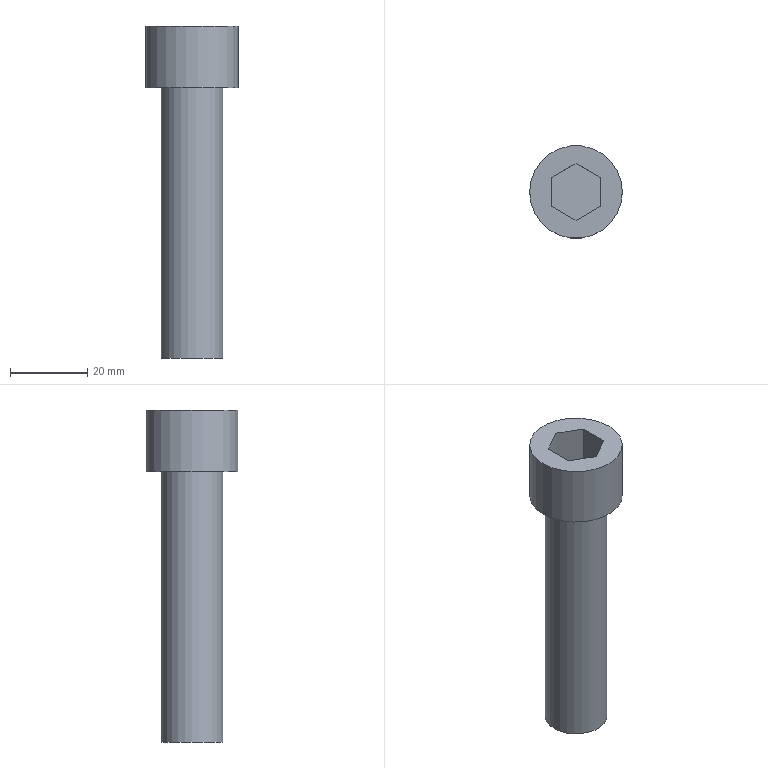Part | NX | features solid 2 | 1 solid | 12 faces | box 24 x 24 x 86 mm | volume 19950 mm3 | plane 10 | cylinder 2 | commonest cylinder face diameters 16 x1 24 x1
STEP:
#1=CARTESIAN_POINT('',(60.4,-707.246,-109.));
#2=VERTEX_POINT('',#1);
#3=CARTESIAN_POINT('',(54.,-710.941,-109.));
#4=VERTEX_POINT('',#3);
#5=CARTESIAN_POINT('',(57.2,-709.094,-109.));
#6=DIRECTION('',(-0.866,-0.5,0.));
#7=VECTOR('',#6,1000.);
#8=LINE('',#5,#7);
#9=EDGE_CURVE('',#2,#4,#8,.T.);
#10=ORIENTED_EDGE('',*,*,#9,.T.);
#11=CARTESIAN_POINT('',(47.6,-707.246,-109.));
#12=VERTEX_POINT('',#11);
#13=CARTESIAN_POINT('',(50.8,-709.094,-109.));
#14=DIRECTION('',(-0.866,0.5,0.));
#15=VECTOR('',#14,1000.);
#16=LINE('',#13,#15);
#17=EDGE_CURVE('',#4,#12,#16,.T.);
#18=ORIENTED_EDGE('',*,*,#17,.T.);
#19=CARTESIAN_POINT('',(47.6,-699.856,-109.));
#20=VERTEX_POINT('',#19);
#21=CARTESIAN_POINT('',(47.6,-703.551,-109.));
#22=DIRECTION('',(0.,1.,0.));
#23=VECTOR('',#22,1000.);
#24=LINE('',#21,#23);
#25=EDGE_CURVE('',#12,#20,#24,.T.);
#26=ORIENTED_EDGE('',*,*,#25,.T.);
#27=CARTESIAN_POINT('',(54.,-696.161,-109.));
#28=VERTEX_POINT('',#27);
#29=CARTESIAN_POINT('',(50.8,-698.009,-109.));
#30=DIRECTION('',(0.866,0.5,0.));
#31=VECTOR('',#30,1000.);
#32=LINE('',#29,#31);
#33=EDGE_CURVE('',#20,#28,#32,.T.);
#34=ORIENTED_EDGE('',*,*,#33,.T.);
#35=CARTESIAN_POINT('',(60.4,-699.856,-109.));
#36=VERTEX_POINT('',#35);
#37=CARTESIAN_POINT('',(57.2,-698.009,-109.));
#38=DIRECTION('',(0.866,-0.5,0.));
#39=VECTOR('',#38,1000.);
#40=LINE('',#37,#39);
#41=EDGE_CURVE('',#28,#36,#40,.T.);
#42=ORIENTED_EDGE('',*,*,#41,.T.);
#43=CARTESIAN_POINT('',(60.4,-703.551,-109.));
#44=DIRECTION('',(0.,-1.,0.));
#45=VECTOR('',#44,1000.);
#46=LINE('',#43,#45);
#47=EDGE_CURVE('',#36,#2,#46,.T.);
#48=ORIENTED_EDGE('',*,*,#47,.T.);
#49=EDGE_LOOP('',(#10,#18,#26,#34,#42,#48));
#50=FACE_BOUND('',#49,.T.);
#51=CARTESIAN_POINT('',(66.,-703.551,-109.));
#52=VERTEX_POINT('',#51);
#53=CARTESIAN_POINT('',(54.,-703.551,-109.));
#54=DIRECTION('',(0.,0.,1.));
#55=DIRECTION('',(1.,0.,0.));
#56=AXIS2_PLACEMENT_3D('',#53,#54,#55);
#57=CIRCLE('',#56,12.);
#58=EDGE_CURVE('',#52,#52,#57,.T.);
#59=ORIENTED_EDGE('',*,*,#58,.T.);
#60=EDGE_LOOP('',(#59));
#61=FACE_BOUND('',#60,.T.);
#62=CARTESIAN_POINT('',(54.,-703.551,-109.));
#63=DIRECTION('',(0.,0.,1.));
#64=DIRECTION('',(-1.,0.,0.));
#65=AXIS2_PLACEMENT_3D('',#62,#63,#64);
#66=PLANE('',#65);
#67=ADVANCED_FACE('',(#50,#61),#66,.T.);
#68=CARTESIAN_POINT('',(62.,-703.551,-125.));
#69=VERTEX_POINT('',#68);
#70=CARTESIAN_POINT('',(54.,-703.551,-125.));
#71=DIRECTION('',(0.,0.,1.));
#72=DIRECTION('',(1.,0.,0.));
#73=AXIS2_PLACEMENT_3D('',#70,#71,#72);
#74=CIRCLE('',#73,8.);
#75=EDGE_CURVE('',#69,#69,#74,.T.);
#76=ORIENTED_EDGE('',*,*,#75,.T.);
#77=EDGE_LOOP('',(#76));
#78=FACE_BOUND('',#77,.T.);
#79=CARTESIAN_POINT('',(42.,-703.551,-125.));
#80=VERTEX_POINT('',#79);
#81=CARTESIAN_POINT('',(54.,-703.551,-125.));
#82=DIRECTION('',(0.,0.,-1.));
#83=DIRECTION('',(-1.,0.,0.));
#84=AXIS2_PLACEMENT_3D('',#81,#82,#83);
#85=CIRCLE('',#84,12.);
#86=EDGE_CURVE('',#80,#80,#85,.T.);
#87=ORIENTED_EDGE('',*,*,#86,.T.);
#88=EDGE_LOOP('',(#87));
#89=FACE_BOUND('',#88,.T.);
#90=CARTESIAN_POINT('',(54.,-703.551,-125.));
#91=DIRECTION('',(0.,0.,-1.));
#92=DIRECTION('',(1.,0.,0.));
#93=AXIS2_PLACEMENT_3D('',#90,#91,#92);
#94=PLANE('',#93);
#95=ADVANCED_FACE('',(#78,#89),#94,.T.);
#96=ORIENTED_EDGE('',*,*,#58,.F.);
#97=EDGE_LOOP('',(#96));
#98=FACE_BOUND('',#97,.T.);
#99=ORIENTED_EDGE('',*,*,#86,.F.);
#100=EDGE_LOOP('',(#99));
#101=FACE_BOUND('',#100,.T.);
#102=CARTESIAN_POINT('',(54.,-703.551,-125.));
#103=DIRECTION('',(0.,0.,1.));
#104=DIRECTION('',(-1.,0.,0.));
#105=AXIS2_PLACEMENT_3D('',#102,#103,#104);
#106=CYLINDRICAL_SURFACE('',#105,12.);
#107=ADVANCED_FACE('',(#98,#101),#106,.T.);
#108=ORIENTED_EDGE('',*,*,#9,.F.);
#109=CARTESIAN_POINT('',(60.4,-707.246,-118.6));
#110=VERTEX_POINT('',#109);
#111=CARTESIAN_POINT('',(60.4,-707.246,-118.6));
#112=DIRECTION('',(0.,0.,1.));
#113=VECTOR('',#112,1000.);
#114=LINE('',#111,#113);
#115=EDGE_CURVE('',#110,#2,#114,.T.);
#116=ORIENTED_EDGE('',*,*,#115,.F.);
#117=CARTESIAN_POINT('',(54.,-710.941,-118.6));
#118=VERTEX_POINT('',#117);
#119=CARTESIAN_POINT('',(60.4,-707.246,-118.6));
#120=DIRECTION('',(-0.866,-0.5,0.));
#121=VECTOR('',#120,1000.);
#122=LINE('',#119,#121);
#123=EDGE_CURVE('',#110,#118,#122,.T.);
#124=ORIENTED_EDGE('',*,*,#123,.T.);
#125=CARTESIAN_POINT('',(54.,-710.941,-118.6));
#126=DIRECTION('',(0.,0.,1.));
#127=VECTOR('',#126,1000.);
#128=LINE('',#125,#127);
#129=EDGE_CURVE('',#118,#4,#128,.T.);
#130=ORIENTED_EDGE('',*,*,#129,.T.);
#131=EDGE_LOOP('',(#108,#116,#124,#130));
#132=FACE_BOUND('',#131,.T.);
#133=CARTESIAN_POINT('',(57.2,-709.094,-110.6));
#134=DIRECTION('',(0.5,-0.866,0.));
#135=DIRECTION('',(-0.866,-0.5,0.));
#136=AXIS2_PLACEMENT_3D('',#133,#134,#135);
#137=PLANE('',#136);
#138=ADVANCED_FACE('',(#132),#137,.F.);
#139=ORIENTED_EDGE('',*,*,#47,.F.);
#140=CARTESIAN_POINT('',(60.4,-699.856,-118.6));
#141=VERTEX_POINT('',#140);
#142=CARTESIAN_POINT('',(60.4,-699.856,-118.6));
#143=DIRECTION('',(0.,0.,1.));
#144=VECTOR('',#143,1000.);
#145=LINE('',#142,#144);
#146=EDGE_CURVE('',#141,#36,#145,.T.);
#147=ORIENTED_EDGE('',*,*,#146,.F.);
#148=CARTESIAN_POINT('',(60.4,-699.856,-118.6));
#149=DIRECTION('',(0.,-1.,0.));
#150=VECTOR('',#149,1000.);
#151=LINE('',#148,#150);
#152=EDGE_CURVE('',#141,#110,#151,.T.);
#153=ORIENTED_EDGE('',*,*,#152,.T.);
#154=ORIENTED_EDGE('',*,*,#115,.T.);
#155=EDGE_LOOP('',(#139,#147,#153,#154));
#156=FACE_BOUND('',#155,.T.);
#157=CARTESIAN_POINT('',(60.4,-703.551,-110.6));
#158=DIRECTION('',(1.,0.,0.));
#159=DIRECTION('',(0.,0.,1.));
#160=AXIS2_PLACEMENT_3D('',#157,#158,#159);
#161=PLANE('',#160);
#162=ADVANCED_FACE('',(#156),#161,.F.);
#163=ORIENTED_EDGE('',*,*,#41,.F.);
#164=CARTESIAN_POINT('',(54.,-696.161,-118.6));
#165=VERTEX_POINT('',#164);
#166=CARTESIAN_POINT('',(54.,-696.161,-118.6));
#167=DIRECTION('',(0.,0.,1.));
#168=VECTOR('',#167,1000.);
#169=LINE('',#166,#168);
#170=EDGE_CURVE('',#165,#28,#169,.T.);
#171=ORIENTED_EDGE('',*,*,#170,.F.);
#172=CARTESIAN_POINT('',(54.,-696.161,-118.6));
#173=DIRECTION('',(0.866,-0.5,0.));
#174=VECTOR('',#173,1000.);
#175=LINE('',#172,#174);
#176=EDGE_CURVE('',#165,#141,#175,.T.);
#177=ORIENTED_EDGE('',*,*,#176,.T.);
#178=ORIENTED_EDGE('',*,*,#146,.T.);
#179=EDGE_LOOP('',(#163,#171,#177,#178));
#180=FACE_BOUND('',#179,.T.);
#181=CARTESIAN_POINT('',(57.2,-698.009,-110.6));
#182=DIRECTION('',(0.5,0.866,0.));
#183=DIRECTION('',(0.866,-0.5,0.));
#184=AXIS2_PLACEMENT_3D('',#181,#182,#183);
#185=PLANE('',#184);
#186=ADVANCED_FACE('',(#180),#185,.F.);
#187=ORIENTED_EDGE('',*,*,#33,.F.);
#188=CARTESIAN_POINT('',(47.6,-699.856,-118.6));
#189=VERTEX_POINT('',#188);
#190=CARTESIAN_POINT('',(47.6,-699.856,-118.6));
#191=DIRECTION('',(0.,0.,1.));
#192=VECTOR('',#191,1000.);
#193=LINE('',#190,#192);
#194=EDGE_CURVE('',#189,#20,#193,.T.);
#195=ORIENTED_EDGE('',*,*,#194,.F.);
#196=CARTESIAN_POINT('',(47.6,-699.856,-118.6));
#197=DIRECTION('',(0.866,0.5,0.));
#198=VECTOR('',#197,1000.);
#199=LINE('',#196,#198);
#200=EDGE_CURVE('',#189,#165,#199,.T.);
#201=ORIENTED_EDGE('',*,*,#200,.T.);
#202=ORIENTED_EDGE('',*,*,#170,.T.);
#203=EDGE_LOOP('',(#187,#195,#201,#202));
#204=FACE_BOUND('',#203,.T.);
#205=CARTESIAN_POINT('',(50.8,-698.009,-110.6));
#206=DIRECTION('',(-0.5,0.866,0.));
#207=DIRECTION('',(0.866,0.5,0.));
#208=AXIS2_PLACEMENT_3D('',#205,#206,#207);
#209=PLANE('',#208);
#210=ADVANCED_FACE('',(#204),#209,.F.);
#211=ORIENTED_EDGE('',*,*,#25,.F.);
#212=CARTESIAN_POINT('',(47.6,-707.246,-118.6));
#213=VERTEX_POINT('',#212);
#214=CARTESIAN_POINT('',(47.6,-707.246,-118.6));
#215=DIRECTION('',(0.,0.,1.));
#216=VECTOR('',#215,1000.);
#217=LINE('',#214,#216);
#218=EDGE_CURVE('',#213,#12,#217,.T.);
#219=ORIENTED_EDGE('',*,*,#218,.F.);
#220=CARTESIAN_POINT('',(47.6,-707.246,-118.6));
#221=DIRECTION('',(0.,1.,0.));
#222=VECTOR('',#221,1000.);
#223=LINE('',#220,#222);
#224=EDGE_CURVE('',#213,#189,#223,.T.);
#225=ORIENTED_EDGE('',*,*,#224,.T.);
#226=ORIENTED_EDGE('',*,*,#194,.T.);
#227=EDGE_LOOP('',(#211,#219,#225,#226));
#228=FACE_BOUND('',#227,.T.);
#229=CARTESIAN_POINT('',(47.6,-703.551,-110.6));
#230=DIRECTION('',(-1.,0.,0.));
#231=DIRECTION('',(0.,0.,-1.));
#232=AXIS2_PLACEMENT_3D('',#229,#230,#231);
#233=PLANE('',#232);
#234=ADVANCED_FACE('',(#228),#233,.F.);
#235=ORIENTED_EDGE('',*,*,#17,.F.);
#236=ORIENTED_EDGE('',*,*,#129,.F.);
#237=CARTESIAN_POINT('',(54.,-710.941,-118.6));
#238=DIRECTION('',(-0.866,0.5,0.));
#239=VECTOR('',#238,1000.);
#240=LINE('',#237,#239);
#241=EDGE_CURVE('',#118,#213,#240,.T.);
#242=ORIENTED_EDGE('',*,*,#241,.T.);
#243=ORIENTED_EDGE('',*,*,#218,.T.);
#244=EDGE_LOOP('',(#235,#236,#242,#243));
#245=FACE_BOUND('',#244,.T.);
#246=CARTESIAN_POINT('',(50.8,-709.094,-110.6));
#247=DIRECTION('',(-0.5,-0.866,0.));
#248=DIRECTION('',(-0.866,0.5,0.));
#249=AXIS2_PLACEMENT_3D('',#246,#247,#248);
#250=PLANE('',#249);
#251=ADVANCED_FACE('',(#245),#250,.F.);
#252=ORIENTED_EDGE('',*,*,#241,.F.);
#253=ORIENTED_EDGE('',*,*,#123,.F.);
#254=ORIENTED_EDGE('',*,*,#152,.F.);
#255=ORIENTED_EDGE('',*,*,#176,.F.);
#256=ORIENTED_EDGE('',*,*,#200,.F.);
#257=ORIENTED_EDGE('',*,*,#224,.F.);
#258=EDGE_LOOP('',(#252,#253,#254,#255,#256,#257));
#259=FACE_BOUND('',#258,.T.);
#260=CARTESIAN_POINT('',(54.,-703.551,-118.6));
#261=DIRECTION('',(0.,0.,-1.));
#262=DIRECTION('',(1.,0.,0.));
#263=AXIS2_PLACEMENT_3D('',#260,#261,#262);
#264=PLANE('',#263);
#265=ADVANCED_FACE('',(#259),#264,.F.);
#266=CARTESIAN_POINT('',(46.,-703.551,-195.));
#267=VERTEX_POINT('',#266);
#268=CARTESIAN_POINT('',(54.,-703.551,-195.));
#269=DIRECTION('',(0.,0.,-1.));
#270=DIRECTION('',(-1.,0.,0.));
#271=AXIS2_PLACEMENT_3D('',#268,#269,#270);
#272=CIRCLE('',#271,8.);
#273=EDGE_CURVE('',#267,#267,#272,.T.);
#274=ORIENTED_EDGE('',*,*,#273,.T.);
#275=EDGE_LOOP('',(#274));
#276=FACE_BOUND('',#275,.T.);
#277=CARTESIAN_POINT('',(54.,-703.551,-195.));
#278=DIRECTION('',(0.,0.,-1.));
#279=DIRECTION('',(1.,0.,0.));
#280=AXIS2_PLACEMENT_3D('',#277,#278,#279);
#281=PLANE('',#280);
#282=ADVANCED_FACE('',(#276),#281,.T.);
#283=ORIENTED_EDGE('',*,*,#273,.F.);
#284=EDGE_LOOP('',(#283));
#285=FACE_BOUND('',#284,.T.);
#286=ORIENTED_EDGE('',*,*,#75,.F.);
#287=EDGE_LOOP('',(#286));
#288=FACE_BOUND('',#287,.T.);
#289=CARTESIAN_POINT('',(54.,-703.551,-125.));
#290=DIRECTION('',(0.,0.,-1.));
#291=DIRECTION('',(1.,0.,0.));
#292=AXIS2_PLACEMENT_3D('',#289,#290,#291);
#293=CYLINDRICAL_SURFACE('',#292,8.);
#294=ADVANCED_FACE('',(#285,#288),#293,.T.);
#295=CLOSED_SHELL('',(#67,#95,#107,#138,#162,#186,#210,#234,#251,#265,#282,#294));
#296=MANIFOLD_SOLID_BREP('',#295);
#297=(LENGTH_UNIT()NAMED_UNIT(*)SI_UNIT(.MILLI.,.METRE.));
#298=UNCERTAINTY_MEASURE_WITH_UNIT(LENGTH_MEASURE(0.00001),#297,'','');
#299=(NAMED_UNIT(*)PLANE_ANGLE_UNIT()SI_UNIT($,.RADIAN.));
#300=(NAMED_UNIT(*)SI_UNIT($,.STERADIAN.)SOLID_ANGLE_UNIT());
#301=(GEOMETRIC_REPRESENTATION_CONTEXT(3)GLOBAL_UNCERTAINTY_ASSIGNED_CONTEXT((#298))GLOBAL_UNIT_ASSIGNED_CONTEXT((#297,#299,#300))REPRESENTATION_CONTEXT('',''));
#302=ADVANCED_BREP_SHAPE_REPRESENTATION('',(#296),#301);